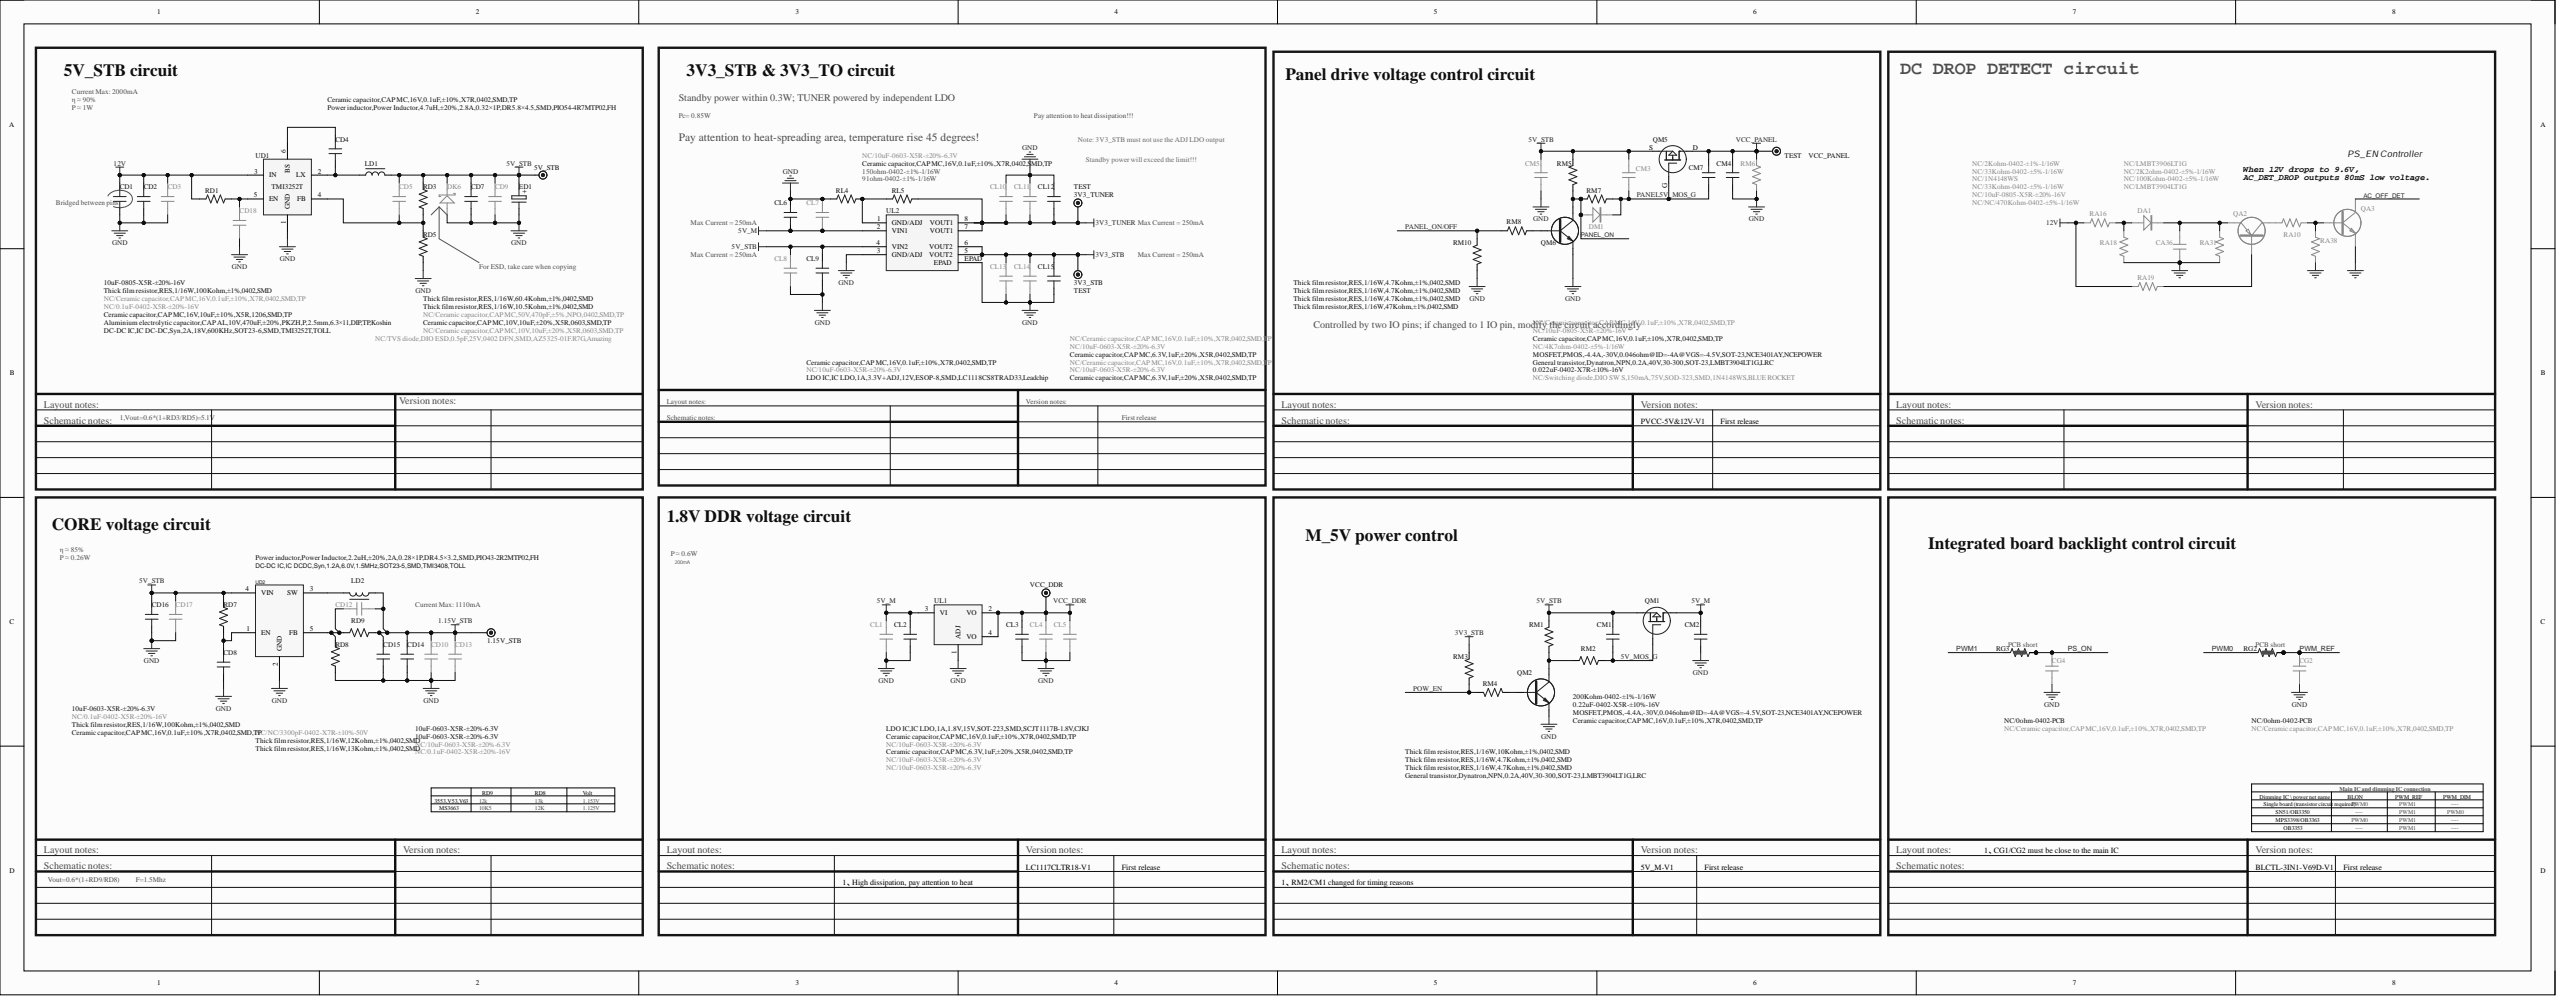Circuit board | Altium Designer | 719 parts | 352 nets | one sheet of the schematic
Parts on this sheet (reference | value | footprint):
1.15V_STB | TEST | TP
3V3_TUNER | TEST | TP
CA36 | NC/10uF-0805-X5R-±20%-16V | C0805
CD1 | Ceramic capacitor,CAP MC,16V,10uF,±10%,X5R,1206,SMD,TP | C1206
CD2 | 10uF-0805-X5R-±20%-16V | C0805
CD3 | NC/Ceramic capacitor,CAP MC,16V,0.1uF,±10%,X7R,0402,SMD,TP | C0402
CD4 | Ceramic capacitor,CAP MC,16V,0.1uF,±10%,X7R,0402,SMD,TP | C0402
CD5 | NC/Ceramic capacitor,CAP MC,50V,470pF,±5%,NPO,0402,SMD,TP | C0402
CD7 | Ceramic capacitor,CAP MC,10V,10uF,±20%,X5R,0603,SMD,TP | C0603
CD8 | Ceramic capacitor,CAP MC,16V,0.1uF,±10%,X7R,0402,SMD,TP | C0402
CD9 | NC/Ceramic capacitor,CAP MC,10V,10uF,±20%,X5R,0603,SMD,TP | C0603
CD10 | NC/10uF-0603-X5R-±20%-6.3V | C0603
CD12 | NC/NC/3300pF-0402-X7R-±10%-50V | C0402
CD13 | NC/0.1uF-0402-X5R-±20%-16V | C0402
CD14 | 10uF-0603-X5R-±20%-6.3V | C0603
CD15 | 10uF-0603-X5R-±20%-6.3V | C0603
CD16 | 10uF-0603-X5R-±20%-6.3V | C0603
CD17 | NC/0.1uF-0402-X5R-±20%-16V | C0402
CD18 | NC/0.1uF-0402-X5R-±20%-16V | C0402
CG2 | NC/Ceramic capacitor,CAP MC,16V,0.1uF,±10%,X7R,0402,SMD,TP | C0402
CG4 | NC/Ceramic capacitor,CAP MC,16V,0.1uF,±10%,X7R,0402,SMD,TP | C0402
CL1 | NC/10uF-0603-X5R-±20%-6.3V | C0603
CL2 | Ceramic capacitor,CAP MC,16V,0.1uF,±10%,X7R,0402,SMD,TP | C0402
CL3 | Ceramic capacitor,CAP MC,6.3V,1uF,±20%,X5R,0402,SMD,TP | C0402
CL4 | NC/10uF-0603-X5R-±20%-6.3V | C0603
CL5 | NC/10uF-0603-X5R-±20%-6.3V | C0603
CL6 | Ceramic capacitor,CAP MC,16V,0.1uF,±10%,X7R,0402,SMD,TP | C0402
CL7 | NC/10uF-0603-X5R-±20%-6.3V | C0603
CL8 | NC/10uF-0603-X5R-±20%-6.3V | C0603
CL9 | Ceramic capacitor,CAP MC,16V,0.1uF,±10%,X7R,0402,SMD,TP | C0402
CL10 | NC/Ceramic capacitor,CAP MC,16V,0.1uF,±10%,X7R,0402,SMD,TP | C0402
CL11 | NC/10uF-0603-X5R-±20%-6.3V | C0603
CL12 | Ceramic capacitor,CAP MC,6.3V,1uF,±20%,X5R,0402,SMD,TP | C0402
CL13 | NC/Ceramic capacitor,CAP MC,16V,0.1uF,±10%,X7R,0402,SMD,TP | C0402
CL14 | NC/10uF-0603-X5R-±20%-6.3V | C0603
CL15 | Ceramic capacitor,CAP MC,6.3V,1uF,±20%,X5R,0402,SMD,TP | C0402
CM1 | 0.22uF-0402-X5R-±10%-16V | C0402
CM2 | Ceramic capacitor,CAP MC,16V,0.1uF,±10%,X7R,0402,SMD,TP | C0402
CM3 | NC/Ceramic capacitor,CAP MC,16V,0.1uF,±10%,X7R,0402,SMD,TP | C0402
CM4 | Ceramic capacitor,CAP MC,16V,0.1uF,±10%,X7R,0402,SMD,TP | C0402
CM5 | NC/10uF-0805-X5R-±20%-16V | C0805
CM7 | 0.022uF-0402-X7R-±10%-16V | C0402
DA1 | NC/1N4148WS | DIODE-S-12
DK6 | NC/TVS diode,DIO ESD,0.5pF,25V,0402 DFN,SMD,AZ5325-01F.R7G,Amazing | DIODE-S0402
DM1 | NC/Switching diode,DIO SW S,150mA,75V,SOD-323,SMD,1N4148WS,BLUE ROCKET | DIODE-S-12
LD1 | Power inductor,Power Inductor,4.7uH,±20%,2.8A,0.32×1P,DR5.8×4.5,SMD,PIO54-4R7MTP02,FH | L(5.8*4.5)-S
LD2 | Power inductor,Power Inductor,2.2uH,±20%,2A,0.28×1P,DR4.5×3.2,SMD,PIO43-2R2MTP02,FH | L(4.5*3.5)-S
PS_ON | TEST | TP_BL
QA2 | NC/LMBT3906LT1G | SOT-23
QA3 | NC/LMBT3904LT1G | SOT-23
QM1 | MOSFET,PMOS,-4.4A,-30V,0.046ohm@ID=-4A@VGS=-4.5V,SOT-23,NCE3401AY,NCEPOWER | SOT-23-1
QM2 | General transistor,Dynatron,NPN,0.2A,40V,30-300,SOT-23,LMBT3904LT1G,LRC | SOT-23
QM5 | MOSFET,PMOS,-4.4A,-30V,0.046ohm@ID=-4A@VGS=-4.5V,SOT-23,NCE3401AY,NCEPOWER | SOT-23-1
QM6 | General transistor,Dynatron,NPN,0.2A,40V,30-300,SOT-23,LMBT3904LT1G,LRC | SOT-23
RA10 | NC/2K2ohm-0402-±5%-1/16W | R0402
RA16 | NC/2Kohm-0402-±1%-1/16W | R0402
RA18 | NC/33Kohm-0402-±5%-1/16W | R0402
RA19 | NC/33Kohm-0402-±5%-1/16W | R0402
RA31 | NC/NC/470Kohm-0402-±5%-1/16W | R0402
RA38 | NC/100Kohm-0402-±5%-1/16W | R0402
RD1 | Thick film resistor,RES,1/16W,100Kohm,±1%,0402,SMD | R0402
RD3 | Thick film resistor,RES,1/16W,60.4Kohm,±1%,0402,SMD | R0402
RD5 | Thick film resistor,RES,1/16W,10.5Kohm,±1%,0402,SMD | R0402
RD7 | Thick film resistor,RES,1/16W,100Kohm,±1%,0402,SMD | R0402
RD8 | Thick film resistor,RES,1/16W,13Kohm,±1%,0402,SMD | R0402
RD9 | Thick film resistor,RES,1/16W,12Kohm,±1%,0402,SMD | R0402
RG2 | NC/0ohm-0402-PCB | R0402SC
RG3 | NC/0ohm-0402-PCB | R0402SC
RL4 | 150ohm-0402-±1%-1/16W | R0402
RL5 | 91ohm-0402-±1%-1/16W | R0402
RM1 | Thick film resistor,RES,1/16W,4.7Kohm,±1%,0402,SMD | R0402
RM2 | 200Kohm-0402-±1%-1/16W | R0402
RM3 | Thick film resistor,RES,1/16W,10Kohm,±1%,0402,SMD | R0402
RM4 | Thick film resistor,RES,1/16W,4.7Kohm,±1%,0402,SMD | R0402
RM5 | Thick film resistor,RES,1/16W,4.7Kohm,±1%,0402,SMD | R0402
RM6 | NC/4K7ohm-0402-±5%-1/16W | R0402
RM7 | Thick film resistor,RES,1/16W,47Kohm,±1%,0402,SMD | R0402
RM8 | Thick film resistor,RES,1/16W,4.7Kohm,±1%,0402,SMD | R0402
RM10 | Thick film resistor,RES,1/16W,4.7Kohm,±1%,0402,SMD | R0402
UD1 | DC-DC IC,IC DC-DC,Syn,2A,18V,600KHz,SOT23-6,SMD,TMI3252T,TOLL | TSOT23-6
UD2 | DC-DC IC,IC DCDC,Syn,1.2A,6.0V,1.5MHz,SOT23-5,SMD,TMI3408,TOLL | SOT-23-5
UL1 | LDO IC,IC LDO,1A,1.8V,15V,SOT-223,SMD,SCJT1117B-1.8V,CJKJ | SOT-223
UL2 | LDO IC,IC LDO,1A,3.3V+ADJ,12V,ESOP-8,SMD,LC1118CS8TRAD33,Leadchip | SOP8/1.27-3
VCC_DDR | TEST | TP
Nets of these parts (net: part-pin ...):
VCC_PANEL: CM4-1 CM7-2 QM5-D RM6-1
VCC_DDR: CL3-2 CL4-2 CL5-2 UL1-2 UL1-4 VCC_DDR-1
PWM_REF: CG2-1 RG2-2 RG2-3
PWM1: RG3-1
PWM0: RG2-1
PS_ON: CG4-1 PS_ON-1 RG3-2 RG3-3
POW_EN: RM3-2 RM4-2
PANEL_ON/OFF: RM8-1 RM10-1
PANEL_ON: DM1-A QM6-C RM5-1 RM7-1
PANEL5V_MOS_G: CM3-1 CM7-1 DM1-K QM5-G RM7-2
NetRL4_2: RL4-2 RL5-1 UL2-1
NetQM6_B: QM6-B RM8-2
NetQM2_C: QM2-C RM1-1 RM2-1
NetQM2_B: QM2-B RM4-1
NetQA3_B: QA3-B RA10-2 RA38-2
NetQA2_C: QA2-C RA10-1
NetQA2_B: QA2-B RA19-1
NetLD2_2: LD2-2 UD2-3
NetDA1_A: DA1-A RA16-2 RA18-2
NetCD18_2: CD18-2 RD1-2 UD1-5
NetCD12_1: CD12-1 RD8-1 RD9-2 UD2-5
NetCD8_2: CD8-2 RD7-1 UD2-1
NetCD5_1: CD5-1 RD3-1 RD5-2 UD1-4
NetCD4_2: CD4-2 UD1-6
NetCD4_1: CD4-1 LD1-1 UD1-2
NetCA36_2: CA36-2 DA1-K QA2-E RA31-2
GND: CA36-1 CD1-1 CD2-2 CD3-1 CD7-1 CD8-1 CD9-1 CD10-1 CD13-1 CD14-1 CD15-1 CD16-1 CD17-1 CD18-1 CG2-2 CG4-2 CL1-1 CL2-1 CL3-1 CL4-1 CL5-1 CL6-1 CL7-1 CL8-1 CL9-1 CL10-1 CL11-2 CL12-1 CL13-2 CL14-2 CL15-2 CM2-2 CM4-2 CM5-1 DK6-A QA3-E QM2-E QM6-E RA18-1 RA31-1 RA38-1 RD5-1 RD8-2 RL4-1 RM6-2 RM10-2 UD1-1 UD2-2 UL1-1 UL2-3 UL2-EPAD
AC_OFF_DET: QA3-C
12V: CD1-2 CD2-1 CD3-2 RA16-1 RA19-2 RD1-1 UD1-3
5V_STB: CD5-2 CD7-2 CD9-2 CD16-2 CD17-2 CL8-2 CL9-2 CM1-1 CM3-2 CM5-2 DK6-K LD1-2 QM1-S QM5-S RD3-2 RD7-2 RM1-2 RM5-2 UD2-4 UL2-4
5V_MOS_G: CM1-2 QM1-G RM2-2
5V_M: CL1-2 CL2-2 CL6-2 CL7-2 CM2-1 QM1-D UL1-3 UL2-2
3V3_TUNER: 3V3_TUNER-1 CL10-2 CL11-1 CL12-2 RL5-2 UL2-7 UL2-8
3V3_STB: CL13-1 CL14-1 CL15-1 RM3-1 UL2-5 UL2-6
1.15V_STB: 1.15V_STB-1 CD10-2 CD12-2 CD13-2 CD14-2 CD15-2 LD2-1 RD9-1